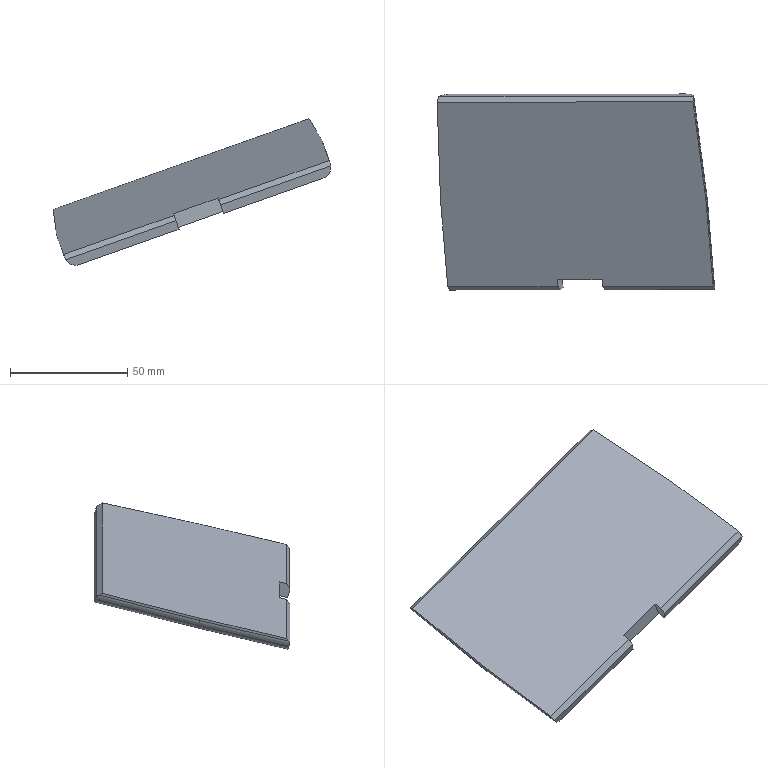Part | STEP file | WEAR-PLATE3_id170_x_t | 1 solid | 19 faces | box 118.359 x 83.443 x 62.371 mm | volume 58708 mm3 | plane 15 | cylinder 4 | commonest cylinder face diameters 10 x4
STEP:
#1=CARTESIAN_POINT('',(109.294,-37.475,-200.15));
#2=VERTEX_POINT('',#1);
#3=CARTESIAN_POINT('',(66.969,-37.475,-215.138));
#4=VERTEX_POINT('',#3);
#5=CARTESIAN_POINT('',(114.007,-37.475,-198.481));
#6=DIRECTION('',(-0.9426,0.,-0.3338));
#7=VECTOR('',#6,1.);
#8=LINE('',#5,#7);
#9=EDGE_CURVE('',#2,#4,#8,.T.);
#10=ORIENTED_EDGE('',*,*,#9,.F.);
#11=CARTESIAN_POINT('',(112.616,-38.443,-194.856));
#12=VERTEX_POINT('',#11);
#13=CARTESIAN_POINT('',(107.674,-38.685,-195.577));
#14=DIRECTION('',(-0.08076,0.9703,0.228));
#15=DIRECTION('',(0.,-0.2288,0.9735));
#16=AXIS2_PLACEMENT_3D('',#13,#14,#15);
#17=CIRCLE('',#16,5.);
#18=EDGE_CURVE('',#12,#2,#17,.T.);
#19=ORIENTED_EDGE('',*,*,#18,.F.);
#20=CARTESIAN_POINT('',(65.674,-38.443,-211.48));
#21=VERTEX_POINT('',#20);
#22=CARTESIAN_POINT('',(65.674,-38.443,-211.48));
#23=DIRECTION('',(0.9426,0.,0.3338));
#24=VECTOR('',#23,1.);
#25=LINE('',#22,#24);
#26=EDGE_CURVE('',#21,#12,#25,.T.);
#27=ORIENTED_EDGE('',*,*,#26,.F.);
#28=CARTESIAN_POINT('',(65.674,-38.443,-211.48));
#29=DIRECTION('',(0.3239,0.2419,-0.9146));
#30=VECTOR('',#29,1.);
#31=LINE('',#28,#30);
#32=EDGE_CURVE('',#21,#4,#31,.T.);
#33=ORIENTED_EDGE('',*,*,#32,.T.);
#34=EDGE_LOOP('',(#10,#19,#27,#33));
#35=FACE_OUTER_BOUND('',#34,.T.);
#36=CARTESIAN_POINT('',(114.007,-37.475,-198.481));
#37=DIRECTION('',(0.08076,-0.9703,-0.228));
#38=DIRECTION('',(0.,0.2288,-0.9735));
#39=AXIS2_PLACEMENT_3D('',#36,#37,#38);
#40=PLANE('',#39);
#41=ADVANCED_FACE('',(#35),#40,.T.);
#42=CARTESIAN_POINT('',(109.189,0.007647,-184.876));
#43=VERTEX_POINT('',#42);
#44=CARTESIAN_POINT('',(109.168,0.,-184.816));
#45=VERTEX_POINT('',#44);
#46=CARTESIAN_POINT('',(109.189,0.007647,-184.876));
#47=CARTESIAN_POINT('',(109.182,0.00255,-184.857));
#48=CARTESIAN_POINT('',(109.175,0.000000502,-184.837));
#49=CARTESIAN_POINT('',(109.168,0.,-184.816));
#50=B_SPLINE_CURVE_WITH_KNOTS('',3,(#46,#47,#48,#49),.UNSPECIFIED.,.F.,.F.,(4,4),(0.,1.),.UNSPECIFIED.);
#51=EDGE_CURVE('',#43,#45,#50,.T.);
#52=ORIENTED_EDGE('',*,*,#51,.T.);
#53=CARTESIAN_POINT('',(112.307,-37.714,-193.68));
#54=VERTEX_POINT('',#53);
#55=CARTESIAN_POINT('',(109.168,0.,-184.816));
#56=DIRECTION('',(0.08076,-0.9703,-0.228));
#57=VECTOR('',#56,1.);
#58=LINE('',#55,#57);
#59=EDGE_CURVE('',#45,#54,#58,.T.);
#60=ORIENTED_EDGE('',*,*,#59,.T.);
#61=CARTESIAN_POINT('',(107.594,-37.714,-195.349));
#62=DIRECTION('',(-0.1719,-0.8572,0.4855));
#63=DIRECTION('',(-0.2861,0.515,0.808));
#64=AXIS2_PLACEMENT_3D('',#61,#62,#63);
#65=ELLIPSE('',#64,7.071,5.);
#66=EDGE_CURVE('',#12,#54,#65,.T.);
#67=ORIENTED_EDGE('',*,*,#66,.F.);
#68=ORIENTED_EDGE('',*,*,#18,.T.);
#69=CARTESIAN_POINT('',(106.085,1.079,-191.089));
#70=VERTEX_POINT('',#69);
#71=CARTESIAN_POINT('',(102.43,45.,-180.766));
#72=DIRECTION('',(0.08076,-0.9703,-0.228));
#73=VECTOR('',#72,1.);
#74=LINE('',#71,#73);
#75=EDGE_CURVE('',#70,#2,#74,.T.);
#76=ORIENTED_EDGE('',*,*,#75,.F.);
#77=CARTESIAN_POINT('',(104.466,-0.1309,-186.516));
#78=DIRECTION('',(-0.1047,0.97,0.2195));
#79=DIRECTION('',(0.9403,0.02465,0.3395));
#80=AXIS2_PLACEMENT_3D('',#77,#78,#79);
#81=ELLIPSE('',#80,5.002,5.);
#82=EDGE_CURVE('',#43,#70,#81,.T.);
#83=ORIENTED_EDGE('',*,*,#82,.F.);
#84=EDGE_LOOP('',(#52,#60,#67,#68,#76,#83));
#85=FACE_OUTER_BOUND('',#84,.T.);
#86=CARTESIAN_POINT('',(107.711,-39.127,-195.681));
#87=DIRECTION('',(-0.08076,0.9703,0.228));
#88=DIRECTION('',(0.,-0.2288,0.9735));
#89=AXIS2_PLACEMENT_3D('',#86,#87,#88);
#90=CYLINDRICAL_SURFACE('',#89,5.);
#91=ADVANCED_FACE('',(#85),#90,.T.);
#92=ORIENTED_EDGE('',*,*,#82,.T.);
#93=CARTESIAN_POINT('',(100.26,45.,-181.535));
#94=VERTEX_POINT('',#93);
#95=CARTESIAN_POINT('',(100.26,45.,-181.535));
#96=DIRECTION('',(0.1285,-0.969,-0.2108));
#97=VECTOR('',#96,1.);
#98=LINE('',#95,#97);
#99=EDGE_CURVE('',#94,#70,#98,.T.);
#100=ORIENTED_EDGE('',*,*,#99,.F.);
#101=CARTESIAN_POINT('',(103.588,44.032,-176.239));
#102=VERTEX_POINT('',#101);
#103=CARTESIAN_POINT('',(98.64,43.79,-176.962));
#104=DIRECTION('',(-0.08076,0.9703,0.228));
#105=DIRECTION('',(0.9426,0.,0.3338));
#106=AXIS2_PLACEMENT_3D('',#103,#104,#105);
#107=ELLIPSE('',#106,5.006,5.);
#108=EDGE_CURVE('',#102,#94,#107,.T.);
#109=ORIENTED_EDGE('',*,*,#108,.F.);
#110=CARTESIAN_POINT('',(103.5,42.897,-175.546));
#111=VERTEX_POINT('',#110);
#112=CARTESIAN_POINT('',(98.769,42.82,-177.173));
#113=DIRECTION('',(0.2861,-0.515,-0.808));
#114=DIRECTION('',(-0.1039,-0.855,0.5082));
#115=AXIS2_PLACEMENT_3D('',#112,#113,#114);
#116=ELLIPSE('',#115,7.08,5.);
#117=EDGE_CURVE('',#102,#111,#116,.T.);
#118=ORIENTED_EDGE('',*,*,#117,.T.);
#119=CARTESIAN_POINT('',(103.5,42.897,-175.546));
#120=DIRECTION('',(0.1285,-0.969,-0.2108));
#121=VECTOR('',#120,1.);
#122=LINE('',#119,#121);
#123=EDGE_CURVE('',#111,#43,#122,.T.);
#124=ORIENTED_EDGE('',*,*,#123,.T.);
#125=EDGE_LOOP('',(#92,#100,#109,#118,#124));
#126=FACE_OUTER_BOUND('',#125,.T.);
#127=CARTESIAN_POINT('',(98.595,44.13,-176.888));
#128=DIRECTION('',(0.1285,-0.969,-0.2108));
#129=DIRECTION('',(0.,0.2126,-0.9771));
#130=AXIS2_PLACEMENT_3D('',#127,#128,#129);
#131=CYLINDRICAL_SURFACE('',#130,5.);
#132=ADVANCED_FACE('',(#126),#131,.T.);
#133=CARTESIAN_POINT('',(0.9088,45.,-216.717));
#134=VERTEX_POINT('',#133);
#135=CARTESIAN_POINT('',(107.143,45.,-179.097));
#136=DIRECTION('',(0.9426,0.,0.3338));
#137=VECTOR('',#136,1.);
#138=LINE('',#135,#137);
#139=EDGE_CURVE('',#134,#94,#138,.T.);
#140=ORIENTED_EDGE('',*,*,#139,.F.);
#141=CARTESIAN_POINT('',(-5.011,44.032,-214.696));
#142=VERTEX_POINT('',#141);
#143=CARTESIAN_POINT('',(-0.7106,43.79,-212.144));
#144=DIRECTION('',(0.08076,-0.9703,-0.228));
#145=DIRECTION('',(0.9426,0.,0.3338));
#146=AXIS2_PLACEMENT_3D('',#143,#144,#145);
#147=ELLIPSE('',#146,5.006,5.);
#148=EDGE_CURVE('',#142,#134,#147,.T.);
#149=ORIENTED_EDGE('',*,*,#148,.F.);
#150=CARTESIAN_POINT('',(103.588,44.032,-176.239));
#151=DIRECTION('',(-0.9426,0.,-0.3338));
#152=VECTOR('',#151,1.);
#153=LINE('',#150,#152);
#154=EDGE_CURVE('',#102,#142,#153,.T.);
#155=ORIENTED_EDGE('',*,*,#154,.F.);
#156=ORIENTED_EDGE('',*,*,#108,.T.);
#157=EDGE_LOOP('',(#140,#149,#155,#156));
#158=FACE_OUTER_BOUND('',#157,.T.);
#159=CARTESIAN_POINT('',(105.847,44.032,-175.439));
#160=DIRECTION('',(-0.08076,0.9703,0.228));
#161=DIRECTION('',(0.,-0.2288,0.9735));
#162=AXIS2_PLACEMENT_3D('',#159,#160,#161);
#163=PLANE('',#162);
#164=ADVANCED_FACE('',(#158),#163,.T.);
#165=CARTESIAN_POINT('',(-3.928,0.007647,-224.932));
#166=VERTEX_POINT('',#165);
#167=CARTESIAN_POINT('',(2.395,1.079,-227.808));
#168=VERTEX_POINT('',#167);
#169=CARTESIAN_POINT('',(0.7751,-0.1309,-223.235));
#170=DIRECTION('',(0.05679,-0.97,-0.2365));
#171=DIRECTION('',(0.9444,-0.02465,0.3279));
#172=AXIS2_PLACEMENT_3D('',#169,#170,#171);
#173=ELLIPSE('',#172,5.002,5.);
#174=EDGE_CURVE('',#166,#168,#173,.T.);
#175=ORIENTED_EDGE('',*,*,#174,.F.);
#176=CARTESIAN_POINT('',(-5.378,42.897,-214.102));
#177=VERTEX_POINT('',#176);
#178=CARTESIAN_POINT('',(-3.928,0.007647,-224.932));
#179=DIRECTION('',(-0.03278,0.969,0.2447));
#180=VECTOR('',#179,1.);
#181=LINE('',#178,#180);
#182=EDGE_CURVE('',#166,#177,#181,.T.);
#183=ORIENTED_EDGE('',*,*,#182,.T.);
#184=CARTESIAN_POINT('',(-0.6778,42.82,-212.389));
#185=DIRECTION('',(-0.2861,0.515,0.808));
#186=DIRECTION('',(0.2391,0.855,-0.4603));
#187=AXIS2_PLACEMENT_3D('',#184,#185,#186);
#188=ELLIPSE('',#187,7.08,5.);
#189=EDGE_CURVE('',#142,#177,#188,.T.);
#190=ORIENTED_EDGE('',*,*,#189,.F.);
#191=ORIENTED_EDGE('',*,*,#148,.T.);
#192=CARTESIAN_POINT('',(2.395,1.079,-227.808));
#193=DIRECTION('',(-0.03278,0.969,0.2447));
#194=VECTOR('',#193,1.);
#195=LINE('',#192,#194);
#196=EDGE_CURVE('',#168,#134,#195,.T.);
#197=ORIENTED_EDGE('',*,*,#196,.F.);
#198=EDGE_LOOP('',(#175,#183,#190,#191,#197));
#199=FACE_OUTER_BOUND('',#198,.T.);
#200=CARTESIAN_POINT('',(2.09,-38.993,-233.048));
#201=DIRECTION('',(-0.03278,0.969,0.2447));
#202=DIRECTION('',(0.,-0.2448,0.9696));
#203=AXIS2_PLACEMENT_3D('',#200,#201,#202);
#204=CYLINDRICAL_SURFACE('',#203,5.);
#205=ADVANCED_FACE('',(#199),#204,.T.);
#206=ORIENTED_EDGE('',*,*,#174,.T.);
#207=CARTESIAN_POINT('',(5.603,-37.475,-236.869));
#208=VERTEX_POINT('',#207);
#209=CARTESIAN_POINT('',(-1.261,45.,-217.485));
#210=DIRECTION('',(-0.08076,0.9703,0.228));
#211=VECTOR('',#210,1.);
#212=LINE('',#209,#211);
#213=EDGE_CURVE('',#208,#168,#212,.T.);
#214=ORIENTED_EDGE('',*,*,#213,.F.);
#215=CARTESIAN_POINT('',(-0.3103,-38.443,-234.846));
#216=VERTEX_POINT('',#215);
#217=CARTESIAN_POINT('',(3.984,-38.685,-232.296));
#218=DIRECTION('',(0.08076,-0.9703,-0.228));
#219=DIRECTION('',(0.,0.2288,-0.9735));
#220=AXIS2_PLACEMENT_3D('',#217,#218,#219);
#221=CIRCLE('',#220,5.);
#222=EDGE_CURVE('',#216,#208,#221,.T.);
#223=ORIENTED_EDGE('',*,*,#222,.F.);
#224=CARTESIAN_POINT('',(-0.8102,-37.714,-233.737));
#225=VERTEX_POINT('',#224);
#226=CARTESIAN_POINT('',(3.903,-37.714,-232.068));
#227=DIRECTION('',(0.1719,0.8572,-0.4855));
#228=DIRECTION('',(0.2861,-0.515,-0.808));
#229=AXIS2_PLACEMENT_3D('',#226,#227,#228);
#230=ELLIPSE('',#229,7.071,5.);
#231=EDGE_CURVE('',#216,#225,#230,.T.);
#232=ORIENTED_EDGE('',*,*,#231,.T.);
#233=CARTESIAN_POINT('',(-3.949,0.,-224.873));
#234=VERTEX_POINT('',#233);
#235=CARTESIAN_POINT('',(-3.949,0.,-224.873));
#236=DIRECTION('',(0.08076,-0.9703,-0.228));
#237=VECTOR('',#236,1.);
#238=LINE('',#235,#237);
#239=EDGE_CURVE('',#234,#225,#238,.T.);
#240=ORIENTED_EDGE('',*,*,#239,.F.);
#241=CARTESIAN_POINT('',(-3.949,0.,-224.873));
#242=CARTESIAN_POINT('',(-3.942,0.000000502,-224.893));
#243=CARTESIAN_POINT('',(-3.935,0.00255,-224.913));
#244=CARTESIAN_POINT('',(-3.928,0.007647,-224.932));
#245=B_SPLINE_CURVE_WITH_KNOTS('',3,(#241,#242,#243,#244),.UNSPECIFIED.,.F.,.F.,(4,4),(0.,1.),.UNSPECIFIED.);
#246=EDGE_CURVE('',#234,#166,#245,.T.);
#247=ORIENTED_EDGE('',*,*,#246,.T.);
#248=EDGE_LOOP('',(#206,#214,#223,#232,#240,#247));
#249=FACE_OUTER_BOUND('',#248,.T.);
#250=CARTESIAN_POINT('',(-2.907,44.105,-212.838));
#251=DIRECTION('',(0.08076,-0.9703,-0.228));
#252=DIRECTION('',(0.,0.2288,-0.9735));
#253=AXIS2_PLACEMENT_3D('',#250,#251,#252);
#254=CYLINDRICAL_SURFACE('',#253,5.);
#255=ADVANCED_FACE('',(#249),#254,.T.);
#256=CARTESIAN_POINT('',(47.928,-37.475,-221.881));
#257=VERTEX_POINT('',#256);
#258=CARTESIAN_POINT('',(5.603,-37.475,-236.869));
#259=DIRECTION('',(0.9426,0.,0.3338));
#260=VECTOR('',#259,1.);
#261=LINE('',#258,#260);
#262=EDGE_CURVE('',#208,#257,#261,.T.);
#263=ORIENTED_EDGE('',*,*,#262,.F.);
#264=ORIENTED_EDGE('',*,*,#213,.T.);
#265=ORIENTED_EDGE('',*,*,#196,.T.);
#266=ORIENTED_EDGE('',*,*,#139,.T.);
#267=ORIENTED_EDGE('',*,*,#99,.T.);
#268=ORIENTED_EDGE('',*,*,#75,.T.);
#269=ORIENTED_EDGE('',*,*,#9,.T.);
#270=CARTESIAN_POINT('',(66.68,-34.,-214.321));
#271=VERTEX_POINT('',#270);
#272=CARTESIAN_POINT('',(66.969,-37.475,-215.138));
#273=DIRECTION('',(-0.08076,0.9703,0.228));
#274=VECTOR('',#273,1.);
#275=LINE('',#272,#274);
#276=EDGE_CURVE('',#4,#271,#275,.T.);
#277=ORIENTED_EDGE('',*,*,#276,.T.);
#278=CARTESIAN_POINT('',(47.639,-34.,-221.064));
#279=VERTEX_POINT('',#278);
#280=CARTESIAN_POINT('',(66.68,-34.,-214.321));
#281=DIRECTION('',(-0.9426,0.,-0.3338));
#282=VECTOR('',#281,1.);
#283=LINE('',#280,#282);
#284=EDGE_CURVE('',#271,#279,#283,.T.);
#285=ORIENTED_EDGE('',*,*,#284,.T.);
#286=CARTESIAN_POINT('',(47.639,-34.,-221.064));
#287=DIRECTION('',(0.08076,-0.9703,-0.228));
#288=VECTOR('',#287,1.);
#289=LINE('',#286,#288);
#290=EDGE_CURVE('',#279,#257,#289,.T.);
#291=ORIENTED_EDGE('',*,*,#290,.T.);
#292=EDGE_LOOP('',(#263,#264,#265,#266,#267,#268,#269,#277,#285,#291));
#293=FACE_OUTER_BOUND('',#292,.T.);
#294=CARTESIAN_POINT('',(107.143,45.,-179.097));
#295=DIRECTION('',(0.3239,0.2419,-0.9146));
#296=DIRECTION('',(-0.9426,0.,-0.3338));
#297=AXIS2_PLACEMENT_3D('',#294,#295,#296);
#298=PLANE('',#297);
#299=ADVANCED_FACE('',(#293),#298,.T.);
#300=CARTESIAN_POINT('',(46.632,-38.443,-218.223));
#301=VERTEX_POINT('',#300);
#302=CARTESIAN_POINT('',(-0.3103,-38.443,-234.846));
#303=DIRECTION('',(0.9426,0.,0.3338));
#304=VECTOR('',#303,1.);
#305=LINE('',#302,#304);
#306=EDGE_CURVE('',#216,#301,#305,.T.);
#307=ORIENTED_EDGE('',*,*,#306,.F.);
#308=ORIENTED_EDGE('',*,*,#222,.T.);
#309=ORIENTED_EDGE('',*,*,#262,.T.);
#310=CARTESIAN_POINT('',(47.928,-37.475,-221.881));
#311=DIRECTION('',(-0.3239,-0.2419,0.9146));
#312=VECTOR('',#311,1.);
#313=LINE('',#310,#312);
#314=EDGE_CURVE('',#257,#301,#313,.T.);
#315=ORIENTED_EDGE('',*,*,#314,.T.);
#316=EDGE_LOOP('',(#307,#308,#309,#315));
#317=FACE_OUTER_BOUND('',#316,.T.);
#318=CARTESIAN_POINT('',(114.007,-37.475,-198.481));
#319=DIRECTION('',(0.08076,-0.9703,-0.228));
#320=DIRECTION('',(0.,0.2288,-0.9735));
#321=AXIS2_PLACEMENT_3D('',#318,#319,#320);
#322=PLANE('',#321);
#323=ADVANCED_FACE('',(#317),#322,.T.);
#324=CARTESIAN_POINT('',(45.574,-34.,-215.235));
#325=VERTEX_POINT('',#324);
#326=CARTESIAN_POINT('',(64.616,-34.,-208.492));
#327=VERTEX_POINT('',#326);
#328=CARTESIAN_POINT('',(111.654,-34.,-191.835));
#329=DIRECTION('',(0.9426,0.,0.3338));
#330=VECTOR('',#329,1.);
#331=LINE('',#328,#330);
#332=EDGE_CURVE('',#325,#327,#331,.T.);
#333=ORIENTED_EDGE('',*,*,#332,.F.);
#334=CARTESIAN_POINT('',(48.138,-34.,-222.475));
#335=DIRECTION('',(0.3338,0.,-0.9426));
#336=VECTOR('',#335,1.);
#337=LINE('',#334,#336);
#338=EDGE_CURVE('',#325,#279,#337,.T.);
#339=ORIENTED_EDGE('',*,*,#338,.T.);
#340=ORIENTED_EDGE('',*,*,#284,.F.);
#341=CARTESIAN_POINT('',(67.179,-34.,-215.732));
#342=DIRECTION('',(-0.3338,0.,0.9426));
#343=VECTOR('',#342,1.);
#344=LINE('',#341,#343);
#345=EDGE_CURVE('',#271,#327,#344,.T.);
#346=ORIENTED_EDGE('',*,*,#345,.T.);
#347=EDGE_LOOP('',(#333,#339,#340,#346));
#348=FACE_OUTER_BOUND('',#347,.T.);
#349=CARTESIAN_POINT('',(48.138,-34.,-222.475));
#350=DIRECTION('',(0.,1.,0.));
#351=DIRECTION('',(0.,0.,1.));
#352=AXIS2_PLACEMENT_3D('',#349,#350,#351);
#353=PLANE('',#352);
#354=ADVANCED_FACE('',(#348),#353,.F.);
#355=CARTESIAN_POINT('',(64.864,-36.986,-209.194));
#356=VERTEX_POINT('',#355);
#357=CARTESIAN_POINT('',(64.864,-36.986,-209.194));
#358=DIRECTION('',(0.2861,-0.515,-0.808));
#359=VECTOR('',#358,1.);
#360=LINE('',#357,#359);
#361=EDGE_CURVE('',#356,#21,#360,.T.);
#362=ORIENTED_EDGE('',*,*,#361,.F.);
#363=CARTESIAN_POINT('',(64.864,-36.986,-209.194));
#364=DIRECTION('',(0.08076,-0.9703,-0.228));
#365=VECTOR('',#364,1.);
#366=LINE('',#363,#365);
#367=EDGE_CURVE('',#327,#356,#366,.T.);
#368=ORIENTED_EDGE('',*,*,#367,.F.);
#369=ORIENTED_EDGE('',*,*,#345,.F.);
#370=ORIENTED_EDGE('',*,*,#276,.F.);
#371=ORIENTED_EDGE('',*,*,#32,.F.);
#372=EDGE_LOOP('',(#362,#368,#369,#370,#371));
#373=FACE_OUTER_BOUND('',#372,.T.);
#374=CARTESIAN_POINT('',(67.179,-34.,-215.732));
#375=DIRECTION('',(0.9426,0.,0.3338));
#376=DIRECTION('',(0.3338,0.,-0.9426));
#377=AXIS2_PLACEMENT_3D('',#374,#375,#376);
#378=PLANE('',#377);
#379=ADVANCED_FACE('',(#373),#378,.F.);
#380=ORIENTED_EDGE('',*,*,#26,.T.);
#381=ORIENTED_EDGE('',*,*,#66,.T.);
#382=CARTESIAN_POINT('',(111.902,-36.986,-192.537));
#383=VERTEX_POINT('',#382);
#384=CARTESIAN_POINT('',(112.307,-37.714,-193.68));
#385=DIRECTION('',(-0.2861,0.515,0.808));
#386=VECTOR('',#385,1.);
#387=LINE('',#384,#386);
#388=EDGE_CURVE('',#54,#383,#387,.T.);
#389=ORIENTED_EDGE('',*,*,#388,.T.);
#390=CARTESIAN_POINT('',(111.902,-36.986,-192.537));
#391=DIRECTION('',(0.9426,0.,0.3338));
#392=VECTOR('',#391,1.);
#393=LINE('',#390,#392);
#394=EDGE_CURVE('',#356,#383,#393,.T.);
#395=ORIENTED_EDGE('',*,*,#394,.F.);
#396=ORIENTED_EDGE('',*,*,#361,.T.);
#397=EDGE_LOOP('',(#380,#381,#389,#395,#396));
#398=FACE_OUTER_BOUND('',#397,.T.);
#399=CARTESIAN_POINT('',(112.711,-38.443,-194.823));
#400=DIRECTION('',(-0.1719,-0.8572,0.4855));
#401=DIRECTION('',(0.,-0.4928,-0.8701));
#402=AXIS2_PLACEMENT_3D('',#399,#400,#401);
#403=PLANE('',#402);
#404=ADVANCED_FACE('',(#398),#403,.T.);
#405=CARTESIAN_POINT('',(108.824,0.,-183.845));
#406=VERTEX_POINT('',#405);
#407=CARTESIAN_POINT('',(111.902,-36.986,-192.537));
#408=DIRECTION('',(-0.08076,0.9703,0.228));
#409=VECTOR('',#408,1.);
#410=LINE('',#407,#409);
#411=EDGE_CURVE('',#383,#406,#410,.T.);
#412=ORIENTED_EDGE('',*,*,#411,.F.);
#413=ORIENTED_EDGE('',*,*,#388,.F.);
#414=ORIENTED_EDGE('',*,*,#59,.F.);
#415=CARTESIAN_POINT('',(50.126,0.,-18.087));
#416=DIRECTION('',(-0.3338,0.,0.9426));
#417=VECTOR('',#416,1.);
#418=LINE('',#415,#417);
#419=EDGE_CURVE('',#45,#406,#418,.T.);
#420=ORIENTED_EDGE('',*,*,#419,.T.);
#421=EDGE_LOOP('',(#412,#413,#414,#420));
#422=FACE_OUTER_BOUND('',#421,.T.);
#423=CARTESIAN_POINT('',(87.012,60.,-122.249));
#424=DIRECTION('',(-0.9426,0.,-0.3338));
#425=DIRECTION('',(-0.3338,0.,0.9426));
#426=AXIS2_PLACEMENT_3D('',#423,#424,#425);
#427=PLANE('',#426);
#428=ADVANCED_FACE('',(#422),#427,.F.);
#429=CARTESIAN_POINT('',(103.305,41.608,-174.793));
#430=VERTEX_POINT('',#429);
#431=CARTESIAN_POINT('',(103.305,41.608,-174.793));
#432=DIRECTION('',(0.1294,0.8563,-0.5));
#433=VECTOR('',#432,1.);
#434=LINE('',#431,#433);
#435=EDGE_CURVE('',#430,#111,#434,.T.);
#436=ORIENTED_EDGE('',*,*,#435,.F.);
#437=CARTESIAN_POINT('',(108.824,0.,-183.845));
#438=DIRECTION('',(-0.1285,0.969,0.2108));
#439=VECTOR('',#438,1.);
#440=LINE('',#437,#439);
#441=EDGE_CURVE('',#406,#430,#440,.T.);
#442=ORIENTED_EDGE('',*,*,#441,.F.);
#443=ORIENTED_EDGE('',*,*,#419,.F.);
#444=ORIENTED_EDGE('',*,*,#51,.F.);
#445=ORIENTED_EDGE('',*,*,#123,.F.);
#446=EDGE_LOOP('',(#436,#442,#443,#444,#445));
#447=FACE_OUTER_BOUND('',#446,.T.);
#448=CARTESIAN_POINT('',(47.162,60.,-19.137));
#449=DIRECTION('',(-0.9413,-0.05234,-0.3333));
#450=DIRECTION('',(-0.3338,0.,0.9426));
#451=AXIS2_PLACEMENT_3D('',#448,#449,#450);
#452=PLANE('',#451);
#453=ADVANCED_FACE('',(#447),#452,.F.);
#454=ORIENTED_EDGE('',*,*,#154,.T.);
#455=ORIENTED_EDGE('',*,*,#189,.T.);
#456=CARTESIAN_POINT('',(-5.7,41.608,-213.395));
#457=VERTEX_POINT('',#456);
#458=CARTESIAN_POINT('',(-5.378,42.897,-214.102));
#459=DIRECTION('',(-0.2141,-0.8563,0.47));
#460=VECTOR('',#459,1.);
#461=LINE('',#458,#460);
#462=EDGE_CURVE('',#177,#457,#461,.T.);
#463=ORIENTED_EDGE('',*,*,#462,.T.);
#464=CARTESIAN_POINT('',(105.361,41.608,-174.066));
#465=DIRECTION('',(-0.9426,0.,-0.3338));
#466=VECTOR('',#465,1.);
#467=LINE('',#464,#466);
#468=EDGE_CURVE('',#430,#457,#467,.T.);
#469=ORIENTED_EDGE('',*,*,#468,.F.);
#470=ORIENTED_EDGE('',*,*,#435,.T.);
#471=ORIENTED_EDGE('',*,*,#117,.F.);
#472=EDGE_LOOP('',(#454,#455,#463,#469,#470,#471));
#473=FACE_OUTER_BOUND('',#472,.T.);
#474=CARTESIAN_POINT('',(105.361,41.608,-174.066));
#475=DIRECTION('',(-0.2861,0.515,0.808));
#476=DIRECTION('',(0.,-0.8433,0.5375));
#477=AXIS2_PLACEMENT_3D('',#474,#475,#476);
#478=PLANE('',#477);
#479=ADVANCED_FACE('',(#473),#478,.T.);
#480=CARTESIAN_POINT('',(-4.293,0.,-223.901));
#481=VERTEX_POINT('',#480);
#482=CARTESIAN_POINT('',(-5.7,41.608,-213.395));
#483=DIRECTION('',(0.03278,-0.969,-0.2447));
#484=VECTOR('',#483,1.);
#485=LINE('',#482,#484);
#486=EDGE_CURVE('',#457,#481,#485,.T.);
#487=ORIENTED_EDGE('',*,*,#486,.F.);
#488=ORIENTED_EDGE('',*,*,#462,.F.);
#489=ORIENTED_EDGE('',*,*,#182,.F.);
#490=ORIENTED_EDGE('',*,*,#246,.F.);
#491=CARTESIAN_POINT('',(-26.105,0.,-162.306));
#492=DIRECTION('',(0.3338,0.,-0.9426));
#493=VECTOR('',#492,1.);
#494=LINE('',#491,#493);
#495=EDGE_CURVE('',#481,#234,#494,.T.);
#496=ORIENTED_EDGE('',*,*,#495,.F.);
#497=EDGE_LOOP('',(#487,#488,#489,#490,#496));
#498=FACE_OUTER_BOUND('',#497,.T.);
#499=CARTESIAN_POINT('',(-62.991,0.,-58.144));
#500=DIRECTION('',(0.9413,-0.05234,0.3333));
#501=DIRECTION('',(0.3338,0.,-0.9426));
#502=AXIS2_PLACEMENT_3D('',#499,#500,#501);
#503=PLANE('',#502);
#504=ADVANCED_FACE('',(#498),#503,.F.);
#505=ORIENTED_EDGE('',*,*,#495,.T.);
#506=ORIENTED_EDGE('',*,*,#239,.T.);
#507=CARTESIAN_POINT('',(-1.215,-36.986,-232.594));
#508=VERTEX_POINT('',#507);
#509=CARTESIAN_POINT('',(-1.215,-36.986,-232.594));
#510=DIRECTION('',(0.2861,-0.515,-0.808));
#511=VECTOR('',#510,1.);
#512=LINE('',#509,#511);
#513=EDGE_CURVE('',#508,#225,#512,.T.);
#514=ORIENTED_EDGE('',*,*,#513,.F.);
#515=CARTESIAN_POINT('',(-1.215,-36.986,-232.594));
#516=DIRECTION('',(0.08076,-0.9703,-0.228));
#517=VECTOR('',#516,1.);
#518=LINE('',#515,#517);
#519=EDGE_CURVE('',#481,#508,#518,.T.);
#520=ORIENTED_EDGE('',*,*,#519,.F.);
#521=EDGE_LOOP('',(#505,#506,#514,#520));
#522=FACE_OUTER_BOUND('',#521,.T.);
#523=CARTESIAN_POINT('',(-26.105,-50.,-162.306));
#524=DIRECTION('',(-0.9426,0.,-0.3338));
#525=DIRECTION('',(-0.3338,0.,0.9426));
#526=AXIS2_PLACEMENT_3D('',#523,#524,#525);
#527=PLANE('',#526);
#528=ADVANCED_FACE('',(#522),#527,.T.);
#529=ORIENTED_EDGE('',*,*,#513,.T.);
#530=ORIENTED_EDGE('',*,*,#231,.F.);
#531=ORIENTED_EDGE('',*,*,#306,.T.);
#532=CARTESIAN_POINT('',(45.823,-36.986,-215.937));
#533=VERTEX_POINT('',#532);
#534=CARTESIAN_POINT('',(46.632,-38.443,-218.223));
#535=DIRECTION('',(-0.2861,0.515,0.808));
#536=VECTOR('',#535,1.);
#537=LINE('',#534,#536);
#538=EDGE_CURVE('',#301,#533,#537,.T.);
#539=ORIENTED_EDGE('',*,*,#538,.T.);
#540=CARTESIAN_POINT('',(111.902,-36.986,-192.537));
#541=DIRECTION('',(0.9426,0.,0.3338));
#542=VECTOR('',#541,1.);
#543=LINE('',#540,#542);
#544=EDGE_CURVE('',#508,#533,#543,.T.);
#545=ORIENTED_EDGE('',*,*,#544,.F.);
#546=EDGE_LOOP('',(#529,#530,#531,#539,#545));
#547=FACE_OUTER_BOUND('',#546,.T.);
#548=CARTESIAN_POINT('',(112.711,-38.443,-194.823));
#549=DIRECTION('',(-0.1719,-0.8572,0.4855));
#550=DIRECTION('',(0.,-0.4928,-0.8701));
#551=AXIS2_PLACEMENT_3D('',#548,#549,#550);
#552=PLANE('',#551);
#553=ADVANCED_FACE('',(#547),#552,.T.);
#554=CARTESIAN_POINT('',(45.823,-36.986,-215.937));
#555=DIRECTION('',(-0.08076,0.9703,0.228));
#556=VECTOR('',#555,1.);
#557=LINE('',#554,#556);
#558=EDGE_CURVE('',#533,#325,#557,.T.);
#559=ORIENTED_EDGE('',*,*,#558,.F.);
#560=ORIENTED_EDGE('',*,*,#538,.F.);
#561=ORIENTED_EDGE('',*,*,#314,.F.);
#562=ORIENTED_EDGE('',*,*,#290,.F.);
#563=ORIENTED_EDGE('',*,*,#338,.F.);
#564=EDGE_LOOP('',(#559,#560,#561,#562,#563));
#565=FACE_OUTER_BOUND('',#564,.T.);
#566=CARTESIAN_POINT('',(48.138,-60.,-222.475));
#567=DIRECTION('',(-0.9426,0.,-0.3338));
#568=DIRECTION('',(-0.3338,0.,0.9426));
#569=AXIS2_PLACEMENT_3D('',#566,#567,#568);
#570=PLANE('',#569);
#571=ADVANCED_FACE('',(#565),#570,.F.);
#572=ORIENTED_EDGE('',*,*,#544,.T.);
#573=ORIENTED_EDGE('',*,*,#558,.T.);
#574=ORIENTED_EDGE('',*,*,#332,.T.);
#575=ORIENTED_EDGE('',*,*,#367,.T.);
#576=ORIENTED_EDGE('',*,*,#394,.T.);
#577=ORIENTED_EDGE('',*,*,#411,.T.);
#578=ORIENTED_EDGE('',*,*,#441,.T.);
#579=ORIENTED_EDGE('',*,*,#468,.T.);
#580=ORIENTED_EDGE('',*,*,#486,.T.);
#581=ORIENTED_EDGE('',*,*,#519,.T.);
#582=EDGE_LOOP('',(#572,#573,#574,#575,#576,#577,#578,#579,#580,#581));
#583=FACE_OUTER_BOUND('',#582,.T.);
#584=CARTESIAN_POINT('',(111.902,-36.986,-192.537));
#585=DIRECTION('',(-0.3239,-0.2419,0.9146));
#586=DIRECTION('',(0.9426,0.,0.3338));
#587=AXIS2_PLACEMENT_3D('',#584,#585,#586);
#588=PLANE('',#587);
#589=ADVANCED_FACE('',(#583),#588,.T.);
#590=CLOSED_SHELL('',(#41,#91,#132,#164,#205,#255,#299,#323,#354,#379,#404,#428,#453,#479,#504,#528,#553,#571,#589));
#591=MANIFOLD_SOLID_BREP('',#590);
#592=(LENGTH_UNIT()NAMED_UNIT(*)SI_UNIT(.MILLI.,.METRE.));
#593=UNCERTAINTY_MEASURE_WITH_UNIT(LENGTH_MEASURE(0.0508),#592,'','');
#594=(NAMED_UNIT(*)PLANE_ANGLE_UNIT()SI_UNIT($,.RADIAN.));
#595=PLANE_ANGLE_MEASURE_WITH_UNIT(PLANE_ANGLE_MEASURE(0.01745),#594);
#596=DIMENSIONAL_EXPONENTS(0.,0.,0.,0.,0.,0.,0.);
#597=(CONVERSION_BASED_UNIT('DEGREE',#595)NAMED_UNIT(#596)PLANE_ANGLE_UNIT());
#598=(NAMED_UNIT(*)SI_UNIT($,.STERADIAN.)SOLID_ANGLE_UNIT());
#599=(GEOMETRIC_REPRESENTATION_CONTEXT(3)GLOBAL_UNCERTAINTY_ASSIGNED_CONTEXT((#593))GLOBAL_UNIT_ASSIGNED_CONTEXT((#592,#597,#598))REPRESENTATION_CONTEXT('',''));
#600=ADVANCED_BREP_SHAPE_REPRESENTATION('',(#591),#599);